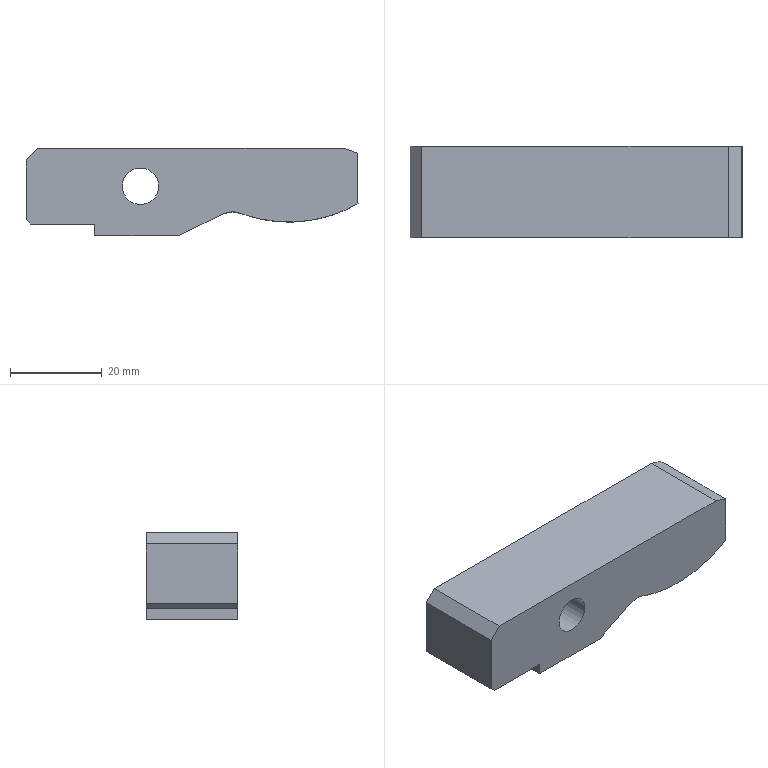Part | 1 solid | 14 faces | box 72.5 x 20 x 19 mm | volume 22819 mm3 | plane 11 | cylinder 2 | other 1 | commonest cylinder face diameters 8 x2
STEP:
#1=CARTESIAN_POINT('',(0.,0.,0.));
#2=DIRECTION('',(0.,0.,1.));
#3=DIRECTION('',(1.,0.,0.));
#4=AXIS2_PLACEMENT_3D('',#1,#2,#3);
#5=CARTESIAN_POINT('',(-58.53,150.526,-242.362));
#6=VERTEX_POINT('',#5);
#7=CARTESIAN_POINT('',(-58.53,150.526,-231.349));
#8=VERTEX_POINT('',#7);
#9=CARTESIAN_POINT('',(-58.53,150.526,-242.362));
#10=DIRECTION('',(-0.000000001,0.,1.));
#11=VECTOR('',#10,1.);
#12=LINE('',#9,#11);
#13=CARTESIAN_POINT('',(-58.53,130.526,-242.362));
#14=DIRECTION('',(-1.,0.,-0.000000001));
#15=DIRECTION('',(0.000000001,0.,-1.));
#16=AXIS2_PLACEMENT_3D('',#13,#14,#15);
#17=PLANE('',#16);
#18=CARTESIAN_POINT('',(0.,-20.));
#19=DIRECTION('',(-1.,0.));
#20=VECTOR('',#19,1.);
#21=LINE('',#18,#20);
#22=(GEOMETRIC_REPRESENTATION_CONTEXT(2)PARAMETRIC_REPRESENTATION_CONTEXT()REPRESENTATION_CONTEXT('',''));
#23=DEFINITIONAL_REPRESENTATION('',(#21),#22);
#24=PCURVE('',#17,#23);
#25=CARTESIAN_POINT('',(-77.88,150.526,-246.104));
#26=DIRECTION('',(0.,-1.,0.));
#27=DIRECTION('',(1.,0.,0.));
#28=AXIS2_PLACEMENT_3D('',#25,#26,#27);
#29=PLANE('',#28);
#30=CARTESIAN_POINT('',(19.35,3.742));
#31=DIRECTION('',(-0.000000001,1.));
#32=VECTOR('',#31,1.);
#33=LINE('',#30,#32);
#34=(GEOMETRIC_REPRESENTATION_CONTEXT(2)PARAMETRIC_REPRESENTATION_CONTEXT()REPRESENTATION_CONTEXT('',''));
#35=DEFINITIONAL_REPRESENTATION('',(#33),#34);
#36=PCURVE('',#29,#35);
#37=SURFACE_CURVE('',#12,(#24,#36),.PCURVE_S1.);
#38=EDGE_CURVE('',#6,#8,#37,.T.);
#39=ORIENTED_EDGE('',*,*,#38,.T.);
#40=CARTESIAN_POINT('',(-58.53,130.526,-231.349));
#41=VERTEX_POINT('',#40);
#42=CARTESIAN_POINT('',(-58.53,130.526,-231.349));
#43=DIRECTION('',(0.,1.,0.));
#44=VECTOR('',#43,1.);
#45=LINE('',#42,#44);
#46=CARTESIAN_POINT('',(-11.013,0.));
#47=DIRECTION('',(0.,-1.));
#48=VECTOR('',#47,1.);
#49=LINE('',#46,#48);
#50=(GEOMETRIC_REPRESENTATION_CONTEXT(2)PARAMETRIC_REPRESENTATION_CONTEXT()REPRESENTATION_CONTEXT('',''));
#51=DEFINITIONAL_REPRESENTATION('',(#49),#50);
#52=PCURVE('',#17,#51);
#53=CARTESIAN_POINT('',(-58.53,130.526,-231.349));
#54=DIRECTION('',(-0.3162,0.,-0.9487));
#55=DIRECTION('',(0.9487,0.,-0.3162));
#56=AXIS2_PLACEMENT_3D('',#53,#54,#55);
#57=PLANE('',#56);
#58=CARTESIAN_POINT('',(0.,0.));
#59=DIRECTION('',(0.,-1.));
#60=VECTOR('',#59,1.);
#61=LINE('',#58,#60);
#62=(GEOMETRIC_REPRESENTATION_CONTEXT(2)PARAMETRIC_REPRESENTATION_CONTEXT()REPRESENTATION_CONTEXT('',''));
#63=DEFINITIONAL_REPRESENTATION('',(#61),#62);
#64=PCURVE('',#57,#63);
#65=SURFACE_CURVE('',#45,(#52,#64),.PCURVE_S1.);
#66=EDGE_CURVE('',#41,#8,#65,.T.);
#67=ORIENTED_EDGE('',*,*,#66,.F.);
#68=CARTESIAN_POINT('',(-58.53,130.526,-242.362));
#69=VERTEX_POINT('',#68);
#70=CARTESIAN_POINT('',(-58.53,130.526,-242.362));
#71=DIRECTION('',(-0.000000001,0.,1.));
#72=VECTOR('',#71,1.);
#73=LINE('',#70,#72);
#74=CARTESIAN_POINT('',(0.,0.));
#75=DIRECTION('',(-1.,0.));
#76=VECTOR('',#75,1.);
#77=LINE('',#74,#76);
#78=(GEOMETRIC_REPRESENTATION_CONTEXT(2)PARAMETRIC_REPRESENTATION_CONTEXT()REPRESENTATION_CONTEXT('',''));
#79=DEFINITIONAL_REPRESENTATION('',(#77),#78);
#80=PCURVE('',#17,#79);
#81=CARTESIAN_POINT('',(-77.88,130.526,-246.104));
#82=DIRECTION('',(0.,-1.,0.));
#83=DIRECTION('',(1.,0.,0.));
#84=AXIS2_PLACEMENT_3D('',#81,#82,#83);
#85=PLANE('',#84);
#86=CARTESIAN_POINT('',(19.35,3.742));
#87=DIRECTION('',(-0.000000001,1.));
#88=VECTOR('',#87,1.);
#89=LINE('',#86,#88);
#90=(GEOMETRIC_REPRESENTATION_CONTEXT(2)PARAMETRIC_REPRESENTATION_CONTEXT()REPRESENTATION_CONTEXT('',''));
#91=DEFINITIONAL_REPRESENTATION('',(#89),#90);
#92=PCURVE('',#85,#91);
#93=SURFACE_CURVE('',#73,(#80,#92),.PCURVE_S1.);
#94=EDGE_CURVE('',#69,#41,#93,.T.);
#95=ORIENTED_EDGE('',*,*,#94,.F.);
#96=CARTESIAN_POINT('',(-58.53,130.526,-242.362));
#97=DIRECTION('',(0.,1.,0.));
#98=VECTOR('',#97,1.);
#99=LINE('',#96,#98);
#100=CARTESIAN_POINT('',(0.,0.));
#101=DIRECTION('',(0.,-1.));
#102=VECTOR('',#101,1.);
#103=LINE('',#100,#102);
#104=(GEOMETRIC_REPRESENTATION_CONTEXT(2)PARAMETRIC_REPRESENTATION_CONTEXT()REPRESENTATION_CONTEXT('',''));
#105=DEFINITIONAL_REPRESENTATION('',(#103),#104);
#106=PCURVE('',#17,#105);
#107=CARTESIAN_POINT('',(-97.53,130.526,-249.349));
#108=CARTESIAN_POINT('',(-94.389,130.526,-247.793));
#109=CARTESIAN_POINT('',(-91.248,130.526,-246.237));
#110=CARTESIAN_POINT('',(-88.106,130.526,-244.681));
#111=CARTESIAN_POINT('',(-86.843,130.526,-244.055));
#112=CARTESIAN_POINT('',(-85.434,130.526,-243.986));
#113=CARTESIAN_POINT('',(-84.116,130.526,-244.486));
#114=CARTESIAN_POINT('',(-75.557,130.526,-247.728));
#115=CARTESIAN_POINT('',(-66.437,130.526,-246.971));
#116=CARTESIAN_POINT('',(-58.53,130.526,-242.362));
#117=(BOUNDED_CURVE()B_SPLINE_CURVE(3,(#107,#108,#109,#110,#111,#112,#113,#114,#115,#116),.UNSPECIFIED.,.F.,.F.)B_SPLINE_CURVE_WITH_KNOTS((4,3,3,4),(0.,2.492,3.494,10.),.UNSPECIFIED.)CURVE()GEOMETRIC_REPRESENTATION_ITEM()RATIONAL_B_SPLINE_CURVE((0.5256,0.5256,0.5256,0.5256,0.4964,0.4964,0.5256,0.4915,0.4915,0.5256))REPRESENTATION_ITEM(''));
#118=DIRECTION('',(0.,1.,0.));
#119=VECTOR('',#118,1.);
#120=SURFACE_OF_LINEAR_EXTRUSION('',#117,#119);
#121=CARTESIAN_POINT('',(10.,0.));
#122=DIRECTION('',(0.,1.));
#123=VECTOR('',#122,1.);
#124=LINE('',#121,#123);
#125=(GEOMETRIC_REPRESENTATION_CONTEXT(2)PARAMETRIC_REPRESENTATION_CONTEXT()REPRESENTATION_CONTEXT('',''));
#126=DEFINITIONAL_REPRESENTATION('',(#124),#125);
#127=PCURVE('',#120,#126);
#128=SURFACE_CURVE('',#99,(#106,#127),.PCURVE_S1.);
#129=EDGE_CURVE('',#69,#6,#128,.T.);
#130=ORIENTED_EDGE('',*,*,#129,.T.);
#131=EDGE_LOOP('',(#39,#67,#95,#130));
#132=FACE_BOUND('',#131,.T.);
#133=ADVANCED_FACE('',(#132),#17,.F.);
#134=CARTESIAN_POINT('',(-97.53,130.526,-249.349));
#135=VERTEX_POINT('',#134);
#136=CARTESIAN_POINT('',(-97.53,150.526,-249.349));
#137=VERTEX_POINT('',#136);
#138=CARTESIAN_POINT('',(-97.53,130.526,-249.349));
#139=DIRECTION('',(0.,1.,0.));
#140=VECTOR('',#139,1.);
#141=LINE('',#138,#140);
#142=CARTESIAN_POINT('',(0.,0.));
#143=DIRECTION('',(0.,1.));
#144=VECTOR('',#143,1.);
#145=LINE('',#142,#144);
#146=(GEOMETRIC_REPRESENTATION_CONTEXT(2)PARAMETRIC_REPRESENTATION_CONTEXT()REPRESENTATION_CONTEXT('',''));
#147=DEFINITIONAL_REPRESENTATION('',(#145),#146);
#148=PCURVE('',#120,#147);
#149=CARTESIAN_POINT('',(-116.03,130.526,-249.349));
#150=DIRECTION('',(0.,0.,1.));
#151=DIRECTION('',(0.,-1.,0.));
#152=AXIS2_PLACEMENT_3D('',#149,#150,#151);
#153=PLANE('',#152);
#154=CARTESIAN_POINT('',(0.,18.5));
#155=DIRECTION('',(-1.,0.));
#156=VECTOR('',#155,1.);
#157=LINE('',#154,#156);
#158=(GEOMETRIC_REPRESENTATION_CONTEXT(2)PARAMETRIC_REPRESENTATION_CONTEXT()REPRESENTATION_CONTEXT('',''));
#159=DEFINITIONAL_REPRESENTATION('',(#157),#158);
#160=PCURVE('',#153,#159);
#161=SURFACE_CURVE('',#141,(#148,#160),.PCURVE_S1.);
#162=EDGE_CURVE('',#135,#137,#161,.T.);
#163=ORIENTED_EDGE('',*,*,#162,.F.);
#164=CARTESIAN_POINT('',(-97.53,130.526,-249.349));
#165=CARTESIAN_POINT('',(-94.389,130.526,-247.793));
#166=CARTESIAN_POINT('',(-91.248,130.526,-246.237));
#167=CARTESIAN_POINT('',(-88.106,130.526,-244.681));
#168=CARTESIAN_POINT('',(-86.843,130.526,-244.055));
#169=CARTESIAN_POINT('',(-85.434,130.526,-243.986));
#170=CARTESIAN_POINT('',(-84.116,130.526,-244.486));
#171=CARTESIAN_POINT('',(-75.557,130.526,-247.728));
#172=CARTESIAN_POINT('',(-66.437,130.526,-246.971));
#173=CARTESIAN_POINT('',(-58.53,130.526,-242.362));
#174=(BOUNDED_CURVE()B_SPLINE_CURVE(3,(#164,#165,#166,#167,#168,#169,#170,#171,#172,#173),.UNSPECIFIED.,.F.,.F.)B_SPLINE_CURVE_WITH_KNOTS((4,3,3,4),(0.,10.129,14.203,42.203),.UNSPECIFIED.)CURVE()GEOMETRIC_REPRESENTATION_ITEM()RATIONAL_B_SPLINE_CURVE((0.5256,0.5256,0.5256,0.5256,0.4964,0.4964,0.5256,0.4915,0.4915,0.5256))REPRESENTATION_ITEM(''));
#175=CARTESIAN_POINT('',(0.,0.));
#176=CARTESIAN_POINT('',(0.1573,0.));
#177=CARTESIAN_POINT('',(0.4719,0.));
#178=CARTESIAN_POINT('',(0.9439,0.));
#179=CARTESIAN_POINT('',(1.416,0.));
#180=CARTESIAN_POINT('',(1.888,0.));
#181=CARTESIAN_POINT('',(2.36,0.));
#182=CARTESIAN_POINT('',(2.831,0.));
#183=CARTESIAN_POINT('',(3.307,0.));
#184=CARTESIAN_POINT('',(3.762,0.));
#185=CARTESIAN_POINT('',(4.205,0.));
#186=CARTESIAN_POINT('',(4.651,0.));
#187=CARTESIAN_POINT('',(5.097,0.));
#188=CARTESIAN_POINT('',(5.543,0.));
#189=CARTESIAN_POINT('',(5.988,0.));
#190=CARTESIAN_POINT('',(6.434,0.));
#191=CARTESIAN_POINT('',(6.88,0.));
#192=CARTESIAN_POINT('',(7.326,0.));
#193=CARTESIAN_POINT('',(7.771,0.));
#194=CARTESIAN_POINT('',(8.217,0.));
#195=CARTESIAN_POINT('',(8.663,0.));
#196=CARTESIAN_POINT('',(9.109,0.));
#197=CARTESIAN_POINT('',(9.554,0.));
#198=CARTESIAN_POINT('',(9.851,0.));
#199=CARTESIAN_POINT('',(10.,0.));
#200=B_SPLINE_CURVE_WITH_KNOTS('',3,(#175,#176,#177,#178,#179,#180,#181,#182,#183,#184,#185,#186,#187,#188,#189,#190,#191,#192,#193,#194,#195,#196,#197,#198,#199),.UNSPECIFIED.,.F.,.F.,(4,1,1,1,1,1,1,1,1,1,1,1,1,1,1,1,1,1,1,1,1,1,4),(0.,1.918,3.837,5.755,7.673,9.592,11.51,13.428,15.346,17.265,19.183,21.101,23.02,24.938,26.856,28.775,30.693,32.611,34.529,36.448,38.366,40.284,42.203),.QUASI_UNIFORM_KNOTS.);
#201=(GEOMETRIC_REPRESENTATION_CONTEXT(2)PARAMETRIC_REPRESENTATION_CONTEXT()REPRESENTATION_CONTEXT('',''));
#202=DEFINITIONAL_REPRESENTATION('',(#200),#201);
#203=PCURVE('',#120,#202);
#204=CARTESIAN_POINT('',(-19.65,-3.245));
#205=CARTESIAN_POINT('',(-16.509,-1.689));
#206=CARTESIAN_POINT('',(-13.368,-0.1328));
#207=CARTESIAN_POINT('',(-10.227,1.423));
#208=CARTESIAN_POINT('',(-8.963,2.049));
#209=CARTESIAN_POINT('',(-7.555,2.118));
#210=CARTESIAN_POINT('',(-6.236,1.618));
#211=CARTESIAN_POINT('',(2.322,-1.624));
#212=CARTESIAN_POINT('',(11.443,-0.867));
#213=CARTESIAN_POINT('',(19.35,3.742));
#214=(BOUNDED_CURVE()B_SPLINE_CURVE(3,(#204,#205,#206,#207,#208,#209,#210,#211,#212,#213),.UNSPECIFIED.,.F.,.F.)B_SPLINE_CURVE_WITH_KNOTS((4,3,3,4),(0.,10.129,14.203,42.203),.UNSPECIFIED.)CURVE()GEOMETRIC_REPRESENTATION_ITEM()RATIONAL_B_SPLINE_CURVE((0.5256,0.5256,0.5256,0.5256,0.4964,0.4964,0.5256,0.4915,0.4915,0.5256))REPRESENTATION_ITEM(''));
#215=(GEOMETRIC_REPRESENTATION_CONTEXT(2)PARAMETRIC_REPRESENTATION_CONTEXT()REPRESENTATION_CONTEXT('',''));
#216=DEFINITIONAL_REPRESENTATION('',(#214),#215);
#217=PCURVE('',#85,#216);
#218=SURFACE_CURVE('',#174,(#203,#217),.PCURVE_S1.);
#219=EDGE_CURVE('',#135,#69,#218,.T.);
#220=ORIENTED_EDGE('',*,*,#219,.T.);
#221=ORIENTED_EDGE('',*,*,#129,.T.);
#222=CARTESIAN_POINT('',(-97.53,150.526,-249.349));
#223=CARTESIAN_POINT('',(-94.389,150.526,-247.793));
#224=CARTESIAN_POINT('',(-91.248,150.526,-246.237));
#225=CARTESIAN_POINT('',(-88.106,150.526,-244.681));
#226=CARTESIAN_POINT('',(-86.843,150.526,-244.055));
#227=CARTESIAN_POINT('',(-85.434,150.526,-243.986));
#228=CARTESIAN_POINT('',(-84.116,150.526,-244.486));
#229=CARTESIAN_POINT('',(-75.557,150.526,-247.728));
#230=CARTESIAN_POINT('',(-66.437,150.526,-246.971));
#231=CARTESIAN_POINT('',(-58.53,150.526,-242.362));
#232=(BOUNDED_CURVE()B_SPLINE_CURVE(3,(#222,#223,#224,#225,#226,#227,#228,#229,#230,#231),.UNSPECIFIED.,.F.,.F.)B_SPLINE_CURVE_WITH_KNOTS((4,3,3,4),(0.,10.129,14.203,42.203),.UNSPECIFIED.)CURVE()GEOMETRIC_REPRESENTATION_ITEM()RATIONAL_B_SPLINE_CURVE((0.5256,0.5256,0.5256,0.5256,0.4964,0.4964,0.5256,0.4915,0.4915,0.5256))REPRESENTATION_ITEM(''));
#233=CARTESIAN_POINT('',(0.,20.));
#234=CARTESIAN_POINT('',(0.1573,20.));
#235=CARTESIAN_POINT('',(0.4719,20.));
#236=CARTESIAN_POINT('',(0.9439,20.));
#237=CARTESIAN_POINT('',(1.416,20.));
#238=CARTESIAN_POINT('',(1.888,20.));
#239=CARTESIAN_POINT('',(2.36,20.));
#240=CARTESIAN_POINT('',(2.831,20.));
#241=CARTESIAN_POINT('',(3.307,20.));
#242=CARTESIAN_POINT('',(3.762,20.));
#243=CARTESIAN_POINT('',(4.205,20.));
#244=CARTESIAN_POINT('',(4.651,20.));
#245=CARTESIAN_POINT('',(5.097,20.));
#246=CARTESIAN_POINT('',(5.543,20.));
#247=CARTESIAN_POINT('',(5.988,20.));
#248=CARTESIAN_POINT('',(6.434,20.));
#249=CARTESIAN_POINT('',(6.88,20.));
#250=CARTESIAN_POINT('',(7.326,20.));
#251=CARTESIAN_POINT('',(7.771,20.));
#252=CARTESIAN_POINT('',(8.217,20.));
#253=CARTESIAN_POINT('',(8.663,20.));
#254=CARTESIAN_POINT('',(9.109,20.));
#255=CARTESIAN_POINT('',(9.554,20.));
#256=CARTESIAN_POINT('',(9.851,20.));
#257=CARTESIAN_POINT('',(10.,20.));
#258=B_SPLINE_CURVE_WITH_KNOTS('',3,(#233,#234,#235,#236,#237,#238,#239,#240,#241,#242,#243,#244,#245,#246,#247,#248,#249,#250,#251,#252,#253,#254,#255,#256,#257),.UNSPECIFIED.,.F.,.F.,(4,1,1,1,1,1,1,1,1,1,1,1,1,1,1,1,1,1,1,1,1,1,4),(0.,1.918,3.837,5.755,7.673,9.592,11.51,13.428,15.346,17.265,19.183,21.101,23.02,24.938,26.856,28.775,30.693,32.611,34.529,36.448,38.366,40.284,42.203),.QUASI_UNIFORM_KNOTS.);
#259=(GEOMETRIC_REPRESENTATION_CONTEXT(2)PARAMETRIC_REPRESENTATION_CONTEXT()REPRESENTATION_CONTEXT('',''));
#260=DEFINITIONAL_REPRESENTATION('',(#258),#259);
#261=PCURVE('',#120,#260);
#262=CARTESIAN_POINT('',(-19.65,-3.245));
#263=CARTESIAN_POINT('',(-16.509,-1.689));
#264=CARTESIAN_POINT('',(-13.368,-0.1328));
#265=CARTESIAN_POINT('',(-10.227,1.423));
#266=CARTESIAN_POINT('',(-8.963,2.049));
#267=CARTESIAN_POINT('',(-7.555,2.118));
#268=CARTESIAN_POINT('',(-6.236,1.618));
#269=CARTESIAN_POINT('',(2.322,-1.624));
#270=CARTESIAN_POINT('',(11.443,-0.867));
#271=CARTESIAN_POINT('',(19.35,3.742));
#272=(BOUNDED_CURVE()B_SPLINE_CURVE(3,(#262,#263,#264,#265,#266,#267,#268,#269,#270,#271),.UNSPECIFIED.,.F.,.F.)B_SPLINE_CURVE_WITH_KNOTS((4,3,3,4),(0.,10.129,14.203,42.203),.UNSPECIFIED.)CURVE()GEOMETRIC_REPRESENTATION_ITEM()RATIONAL_B_SPLINE_CURVE((0.5256,0.5256,0.5256,0.5256,0.4964,0.4964,0.5256,0.4915,0.4915,0.5256))REPRESENTATION_ITEM(''));
#273=(GEOMETRIC_REPRESENTATION_CONTEXT(2)PARAMETRIC_REPRESENTATION_CONTEXT()REPRESENTATION_CONTEXT('',''));
#274=DEFINITIONAL_REPRESENTATION('',(#272),#273);
#275=PCURVE('',#29,#274);
#276=SURFACE_CURVE('',#232,(#261,#275),.PCURVE_S1.);
#277=EDGE_CURVE('',#137,#6,#276,.T.);
#278=ORIENTED_EDGE('',*,*,#277,.F.);
#279=EDGE_LOOP('',(#163,#220,#221,#278));
#280=FACE_BOUND('',#279,.F.);
#281=ADVANCED_FACE('',(#280),#120,.F.);
#282=CARTESIAN_POINT('',(-116.03,150.526,-249.349));
#283=VERTEX_POINT('',#282);
#284=CARTESIAN_POINT('',(-116.03,150.526,-249.349));
#285=DIRECTION('',(1.,0.,0.));
#286=VECTOR('',#285,1.);
#287=LINE('',#284,#286);
#288=CARTESIAN_POINT('',(-20.,0.));
#289=DIRECTION('',(0.,1.));
#290=VECTOR('',#289,1.);
#291=LINE('',#288,#290);
#292=(GEOMETRIC_REPRESENTATION_CONTEXT(2)PARAMETRIC_REPRESENTATION_CONTEXT()REPRESENTATION_CONTEXT('',''));
#293=DEFINITIONAL_REPRESENTATION('',(#291),#292);
#294=PCURVE('',#153,#293);
#295=CARTESIAN_POINT('',(-38.15,-3.245));
#296=DIRECTION('',(1.,0.));
#297=VECTOR('',#296,1.);
#298=LINE('',#295,#297);
#299=(GEOMETRIC_REPRESENTATION_CONTEXT(2)PARAMETRIC_REPRESENTATION_CONTEXT()REPRESENTATION_CONTEXT('',''));
#300=DEFINITIONAL_REPRESENTATION('',(#298),#299);
#301=PCURVE('',#29,#300);
#302=SURFACE_CURVE('',#287,(#294,#301),.PCURVE_S1.);
#303=EDGE_CURVE('',#283,#137,#302,.T.);
#304=ORIENTED_EDGE('',*,*,#303,.T.);
#305=ORIENTED_EDGE('',*,*,#162,.F.);
#306=CARTESIAN_POINT('',(-116.03,130.526,-249.349));
#307=VERTEX_POINT('',#306);
#308=CARTESIAN_POINT('',(-116.03,130.526,-249.349));
#309=DIRECTION('',(1.,0.,0.));
#310=VECTOR('',#309,1.);
#311=LINE('',#308,#310);
#312=CARTESIAN_POINT('',(0.,0.));
#313=DIRECTION('',(0.,1.));
#314=VECTOR('',#313,1.);
#315=LINE('',#312,#314);
#316=(GEOMETRIC_REPRESENTATION_CONTEXT(2)PARAMETRIC_REPRESENTATION_CONTEXT()REPRESENTATION_CONTEXT('',''));
#317=DEFINITIONAL_REPRESENTATION('',(#315),#316);
#318=PCURVE('',#153,#317);
#319=CARTESIAN_POINT('',(-38.15,-3.245));
#320=DIRECTION('',(1.,0.));
#321=VECTOR('',#320,1.);
#322=LINE('',#319,#321);
#323=(GEOMETRIC_REPRESENTATION_CONTEXT(2)PARAMETRIC_REPRESENTATION_CONTEXT()REPRESENTATION_CONTEXT('',''));
#324=DEFINITIONAL_REPRESENTATION('',(#322),#323);
#325=PCURVE('',#85,#324);
#326=SURFACE_CURVE('',#311,(#318,#325),.PCURVE_S1.);
#327=EDGE_CURVE('',#307,#135,#326,.T.);
#328=ORIENTED_EDGE('',*,*,#327,.F.);
#329=CARTESIAN_POINT('',(-116.03,130.526,-249.349));
#330=DIRECTION('',(0.,1.,0.));
#331=VECTOR('',#330,1.);
#332=LINE('',#329,#331);
#333=CARTESIAN_POINT('',(0.,0.));
#334=DIRECTION('',(-1.,0.));
#335=VECTOR('',#334,1.);
#336=LINE('',#333,#335);
#337=(GEOMETRIC_REPRESENTATION_CONTEXT(2)PARAMETRIC_REPRESENTATION_CONTEXT()REPRESENTATION_CONTEXT('',''));
#338=DEFINITIONAL_REPRESENTATION('',(#336),#337);
#339=PCURVE('',#153,#338);
#340=CARTESIAN_POINT('',(-116.03,130.526,-246.849));
#341=DIRECTION('',(1.,0.,0.));
#342=DIRECTION('',(0.,0.,1.));
#343=AXIS2_PLACEMENT_3D('',#340,#341,#342);
#344=PLANE('',#343);
#345=CARTESIAN_POINT('',(-2.5,0.));
#346=DIRECTION('',(0.,-1.));
#347=VECTOR('',#346,1.);
#348=LINE('',#345,#347);
#349=(GEOMETRIC_REPRESENTATION_CONTEXT(2)PARAMETRIC_REPRESENTATION_CONTEXT()REPRESENTATION_CONTEXT('',''));
#350=DEFINITIONAL_REPRESENTATION('',(#348),#349);
#351=PCURVE('',#344,#350);
#352=SURFACE_CURVE('',#332,(#339,#351),.PCURVE_S1.);
#353=EDGE_CURVE('',#307,#283,#352,.T.);
#354=ORIENTED_EDGE('',*,*,#353,.T.);
#355=EDGE_LOOP('',(#304,#305,#328,#354));
#356=FACE_BOUND('',#355,.T.);
#357=ADVANCED_FACE('',(#356),#153,.F.);
#358=CARTESIAN_POINT('',(-116.03,150.526,-246.849));
#359=VERTEX_POINT('',#358);
#360=CARTESIAN_POINT('',(-116.03,150.526,-246.849));
#361=DIRECTION('',(0.,0.,-1.));
#362=VECTOR('',#361,1.);
#363=LINE('',#360,#362);
#364=CARTESIAN_POINT('',(0.,-20.));
#365=DIRECTION('',(-1.,0.));
#366=VECTOR('',#365,1.);
#367=LINE('',#364,#366);
#368=(GEOMETRIC_REPRESENTATION_CONTEXT(2)PARAMETRIC_REPRESENTATION_CONTEXT()REPRESENTATION_CONTEXT('',''));
#369=DEFINITIONAL_REPRESENTATION('',(#367),#368);
#370=PCURVE('',#344,#369);
#371=CARTESIAN_POINT('',(-38.15,-0.7447));
#372=DIRECTION('',(0.,-1.));
#373=VECTOR('',#372,1.);
#374=LINE('',#371,#373);
#375=(GEOMETRIC_REPRESENTATION_CONTEXT(2)PARAMETRIC_REPRESENTATION_CONTEXT()REPRESENTATION_CONTEXT('',''));
#376=DEFINITIONAL_REPRESENTATION('',(#374),#375);
#377=PCURVE('',#29,#376);
#378=SURFACE_CURVE('',#363,(#370,#377),.PCURVE_S1.);
#379=EDGE_CURVE('',#359,#283,#378,.T.);
#380=ORIENTED_EDGE('',*,*,#379,.T.);
#381=ORIENTED_EDGE('',*,*,#353,.F.);
#382=CARTESIAN_POINT('',(-116.03,130.526,-246.849));
#383=VERTEX_POINT('',#382);
#384=CARTESIAN_POINT('',(-116.03,130.526,-246.849));
#385=DIRECTION('',(0.,0.,-1.));
#386=VECTOR('',#385,1.);
#387=LINE('',#384,#386);
#388=CARTESIAN_POINT('',(0.,0.));
#389=DIRECTION('',(-1.,0.));
#390=VECTOR('',#389,1.);
#391=LINE('',#388,#390);
#392=(GEOMETRIC_REPRESENTATION_CONTEXT(2)PARAMETRIC_REPRESENTATION_CONTEXT()REPRESENTATION_CONTEXT('',''));
#393=DEFINITIONAL_REPRESENTATION('',(#391),#392);
#394=PCURVE('',#344,#393);
#395=CARTESIAN_POINT('',(-38.15,-0.7447));
#396=DIRECTION('',(0.,-1.));
#397=VECTOR('',#396,1.);
#398=LINE('',#395,#397);
#399=(GEOMETRIC_REPRESENTATION_CONTEXT(2)PARAMETRIC_REPRESENTATION_CONTEXT()REPRESENTATION_CONTEXT('',''));
#400=DEFINITIONAL_REPRESENTATION('',(#398),#399);
#401=PCURVE('',#85,#400);
#402=SURFACE_CURVE('',#387,(#394,#401),.PCURVE_S1.);
#403=EDGE_CURVE('',#383,#307,#402,.T.);
#404=ORIENTED_EDGE('',*,*,#403,.F.);
#405=CARTESIAN_POINT('',(-116.03,130.526,-246.849));
#406=DIRECTION('',(0.,1.,0.));
#407=VECTOR('',#406,1.);
#408=LINE('',#405,#407);
#409=CARTESIAN_POINT('',(0.,0.));
#410=DIRECTION('',(0.,-1.));
#411=VECTOR('',#410,1.);
#412=LINE('',#409,#411);
#413=(GEOMETRIC_REPRESENTATION_CONTEXT(2)PARAMETRIC_REPRESENTATION_CONTEXT()REPRESENTATION_CONTEXT('',''));
#414=DEFINITIONAL_REPRESENTATION('',(#412),#413);
#415=PCURVE('',#344,#414);
#416=CARTESIAN_POINT('',(-130.03,130.526,-246.849));
#417=DIRECTION('',(0.,0.,1.));
#418=DIRECTION('',(-1.,0.,0.));
#419=AXIS2_PLACEMENT_3D('',#416,#417,#418);
#420=PLANE('',#419);
#421=CARTESIAN_POINT('',(-14.,0.));
#422=DIRECTION('',(0.,-1.));
#423=VECTOR('',#422,1.);
#424=LINE('',#421,#423);
#425=(GEOMETRIC_REPRESENTATION_CONTEXT(2)PARAMETRIC_REPRESENTATION_CONTEXT()REPRESENTATION_CONTEXT('',''));
#426=DEFINITIONAL_REPRESENTATION('',(#424),#425);
#427=PCURVE('',#420,#426);
#428=SURFACE_CURVE('',#408,(#415,#427),.PCURVE_S1.);
#429=EDGE_CURVE('',#383,#359,#428,.T.);
#430=ORIENTED_EDGE('',*,*,#429,.T.);
#431=EDGE_LOOP('',(#380,#381,#404,#430));
#432=FACE_BOUND('',#431,.T.);
#433=ADVANCED_FACE('',(#432),#344,.F.);
#434=CARTESIAN_POINT('',(-130.03,150.526,-246.849));
#435=VERTEX_POINT('',#434);
#436=CARTESIAN_POINT('',(-130.03,150.526,-246.849));
#437=DIRECTION('',(1.,0.,0.));
#438=VECTOR('',#437,1.);
#439=LINE('',#436,#438);
#440=CARTESIAN_POINT('',(0.,-20.));
#441=DIRECTION('',(-1.,0.));
#442=VECTOR('',#441,1.);
#443=LINE('',#440,#442);
#444=(GEOMETRIC_REPRESENTATION_CONTEXT(2)PARAMETRIC_REPRESENTATION_CONTEXT()REPRESENTATION_CONTEXT('',''));
#445=DEFINITIONAL_REPRESENTATION('',(#443),#444);
#446=PCURVE('',#420,#445);
#447=CARTESIAN_POINT('',(-52.15,-0.7447));
#448=DIRECTION('',(1.,0.));
#449=VECTOR('',#448,1.);
#450=LINE('',#447,#449);
#451=(GEOMETRIC_REPRESENTATION_CONTEXT(2)PARAMETRIC_REPRESENTATION_CONTEXT()REPRESENTATION_CONTEXT('',''));
#452=DEFINITIONAL_REPRESENTATION('',(#450),#451);
#453=PCURVE('',#29,#452);
#454=SURFACE_CURVE('',#439,(#446,#453),.PCURVE_S1.);
#455=EDGE_CURVE('',#435,#359,#454,.T.);
#456=ORIENTED_EDGE('',*,*,#455,.T.);
#457=ORIENTED_EDGE('',*,*,#429,.F.);
#458=CARTESIAN_POINT('',(-130.03,130.526,-246.849));
#459=VERTEX_POINT('',#458);
#460=CARTESIAN_POINT('',(-130.03,130.526,-246.849));
#461=DIRECTION('',(1.,0.,0.));
#462=VECTOR('',#461,1.);
#463=LINE('',#460,#462);
#464=CARTESIAN_POINT('',(0.,0.));
#465=DIRECTION('',(-1.,0.));
#466=VECTOR('',#465,1.);
#467=LINE('',#464,#466);
#468=(GEOMETRIC_REPRESENTATION_CONTEXT(2)PARAMETRIC_REPRESENTATION_CONTEXT()REPRESENTATION_CONTEXT('',''));
#469=DEFINITIONAL_REPRESENTATION('',(#467),#468);
#470=PCURVE('',#420,#469);
#471=CARTESIAN_POINT('',(-52.15,-0.7447));
#472=DIRECTION('',(1.,0.));
#473=VECTOR('',#472,1.);
#474=LINE('',#471,#473);
#475=(GEOMETRIC_REPRESENTATION_CONTEXT(2)PARAMETRIC_REPRESENTATION_CONTEXT()REPRESENTATION_CONTEXT('',''));
#476=DEFINITIONAL_REPRESENTATION('',(#474),#475);
#477=PCURVE('',#85,#476);
#478=SURFACE_CURVE('',#463,(#470,#477),.PCURVE_S1.);
#479=EDGE_CURVE('',#459,#383,#478,.T.);
#480=ORIENTED_EDGE('',*,*,#479,.F.);
#481=CARTESIAN_POINT('',(-130.03,130.526,-246.849));
#482=DIRECTION('',(0.,1.,0.));
#483=VECTOR('',#482,1.);
#484=LINE('',#481,#483);
#485=CARTESIAN_POINT('',(0.,0.));
#486=DIRECTION('',(0.,-1.));
#487=VECTOR('',#486,1.);
#488=LINE('',#485,#487);
#489=(GEOMETRIC_REPRESENTATION_CONTEXT(2)PARAMETRIC_REPRESENTATION_CONTEXT()REPRESENTATION_CONTEXT('',''));
#490=DEFINITIONAL_REPRESENTATION('',(#488),#489);
#491=PCURVE('',#420,#490);
#492=CARTESIAN_POINT('',(-131.03,130.526,-245.849));
#493=DIRECTION('',(0.7071,0.,0.7071));
#494=DIRECTION('',(-0.7071,0.,0.7071));
#495=AXIS2_PLACEMENT_3D('',#492,#493,#494);
#496=PLANE('',#495);
#497=CARTESIAN_POINT('',(-1.414,0.));
#498=DIRECTION('',(0.,-1.));
#499=VECTOR('',#498,1.);
#500=LINE('',#497,#499);
#501=(GEOMETRIC_REPRESENTATION_CONTEXT(2)PARAMETRIC_REPRESENTATION_CONTEXT()REPRESENTATION_CONTEXT('',''));
#502=DEFINITIONAL_REPRESENTATION('',(#500),#501);
#503=PCURVE('',#496,#502);
#504=SURFACE_CURVE('',#484,(#491,#503),.PCURVE_S1.);
#505=EDGE_CURVE('',#459,#435,#504,.T.);
#506=ORIENTED_EDGE('',*,*,#505,.T.);
#507=EDGE_LOOP('',(#456,#457,#480,#506));
#508=FACE_BOUND('',#507,.T.);
#509=ADVANCED_FACE('',(#508),#420,.F.);
#510=CARTESIAN_POINT('',(-131.03,150.526,-245.849));
#511=VERTEX_POINT('',#510);
#512=CARTESIAN_POINT('',(-131.03,150.526,-245.849));
#513=DIRECTION('',(0.7071,0.,-0.7071));
#514=VECTOR('',#513,1.);
#515=LINE('',#512,#514);
#516=CARTESIAN_POINT('',(0.,-20.));
#517=DIRECTION('',(-1.,0.));
#518=VECTOR('',#517,1.);
#519=LINE('',#516,#518);
#520=(GEOMETRIC_REPRESENTATION_CONTEXT(2)PARAMETRIC_REPRESENTATION_CONTEXT()REPRESENTATION_CONTEXT('',''));
#521=DEFINITIONAL_REPRESENTATION('',(#519),#520);
#522=PCURVE('',#496,#521);
#523=CARTESIAN_POINT('',(-53.15,0.2553));
#524=DIRECTION('',(0.7071,-0.7071));
#525=VECTOR('',#524,1.);
#526=LINE('',#523,#525);
#527=(GEOMETRIC_REPRESENTATION_CONTEXT(2)PARAMETRIC_REPRESENTATION_CONTEXT()REPRESENTATION_CONTEXT('',''));
#528=DEFINITIONAL_REPRESENTATION('',(#526),#527);
#529=PCURVE('',#29,#528);
#530=SURFACE_CURVE('',#515,(#522,#529),.PCURVE_S1.);
#531=EDGE_CURVE('',#511,#435,#530,.T.);
#532=ORIENTED_EDGE('',*,*,#531,.T.);
#533=ORIENTED_EDGE('',*,*,#505,.F.);
#534=CARTESIAN_POINT('',(-131.03,130.526,-245.849));
#535=VERTEX_POINT('',#534);
#536=CARTESIAN_POINT('',(-131.03,130.526,-245.849));
#537=DIRECTION('',(0.7071,0.,-0.7071));
#538=VECTOR('',#537,1.);
#539=LINE('',#536,#538);
#540=CARTESIAN_POINT('',(0.,0.));
#541=DIRECTION('',(-1.,0.));
#542=VECTOR('',#541,1.);
#543=LINE('',#540,#542);
#544=(GEOMETRIC_REPRESENTATION_CONTEXT(2)PARAMETRIC_REPRESENTATION_CONTEXT()REPRESENTATION_CONTEXT('',''));
#545=DEFINITIONAL_REPRESENTATION('',(#543),#544);
#546=PCURVE('',#496,#545);
#547=CARTESIAN_POINT('',(-53.15,0.2553));
#548=DIRECTION('',(0.7071,-0.7071));
#549=VECTOR('',#548,1.);
#550=LINE('',#547,#549);
#551=(GEOMETRIC_REPRESENTATION_CONTEXT(2)PARAMETRIC_REPRESENTATION_CONTEXT()REPRESENTATION_CONTEXT('',''));
#552=DEFINITIONAL_REPRESENTATION('',(#550),#551);
#553=PCURVE('',#85,#552);
#554=SURFACE_CURVE('',#539,(#546,#553),.PCURVE_S1.);
#555=EDGE_CURVE('',#535,#459,#554,.T.);
#556=ORIENTED_EDGE('',*,*,#555,.F.);
#557=CARTESIAN_POINT('',(-131.03,130.526,-245.849));
#558=DIRECTION('',(0.,1.,0.));
#559=VECTOR('',#558,1.);
#560=LINE('',#557,#559);
#561=CARTESIAN_POINT('',(0.,0.));
#562=DIRECTION('',(0.,-1.));
#563=VECTOR('',#562,1.);
#564=LINE('',#561,#563);
#565=(GEOMETRIC_REPRESENTATION_CONTEXT(2)PARAMETRIC_REPRESENTATION_CONTEXT()REPRESENTATION_CONTEXT('',''));
#566=DEFINITIONAL_REPRESENTATION('',(#564),#565);
#567=PCURVE('',#496,#566);
#568=CARTESIAN_POINT('',(-131.03,130.526,-232.849));
#569=DIRECTION('',(1.,0.,0.));
#570=DIRECTION('',(0.,1.,0.));
#571=AXIS2_PLACEMENT_3D('',#568,#569,#570);
#572=PLANE('',#571);
#573=CARTESIAN_POINT('',(0.,-13.));
#574=DIRECTION('',(1.,0.));
#575=VECTOR('',#574,1.);
#576=LINE('',#573,#575);
#577=(GEOMETRIC_REPRESENTATION_CONTEXT(2)PARAMETRIC_REPRESENTATION_CONTEXT()REPRESENTATION_CONTEXT('',''));
#578=DEFINITIONAL_REPRESENTATION('',(#576),#577);
#579=PCURVE('',#572,#578);
#580=SURFACE_CURVE('',#560,(#567,#579),.PCURVE_S1.);
#581=EDGE_CURVE('',#535,#511,#580,.T.);
#582=ORIENTED_EDGE('',*,*,#581,.T.);
#583=EDGE_LOOP('',(#532,#533,#556,#582));
#584=FACE_BOUND('',#583,.T.);
#585=ADVANCED_FACE('',(#584),#496,.F.);
#586=CARTESIAN_POINT('',(-131.03,150.526,-232.849));
#587=VERTEX_POINT('',#586);
#588=CARTESIAN_POINT('',(-131.03,150.526,-232.849));
#589=DIRECTION('',(0.,0.,-1.));
#590=VECTOR('',#589,1.);
#591=LINE('',#588,#590);
#592=CARTESIAN_POINT('',(20.,0.));
#593=DIRECTION('',(0.,-1.));
#594=VECTOR('',#593,1.);
#595=LINE('',#592,#594);
#596=(GEOMETRIC_REPRESENTATION_CONTEXT(2)PARAMETRIC_REPRESENTATION_CONTEXT()REPRESENTATION_CONTEXT('',''));
#597=DEFINITIONAL_REPRESENTATION('',(#595),#596);
#598=PCURVE('',#572,#597);
#599=CARTESIAN_POINT('',(-53.15,13.255));
#600=DIRECTION('',(0.,-1.));
#601=VECTOR('',#600,1.);
#602=LINE('',#599,#601);
#603=(GEOMETRIC_REPRESENTATION_CONTEXT(2)PARAMETRIC_REPRESENTATION_CONTEXT()REPRESENTATION_CONTEXT('',''));
#604=DEFINITIONAL_REPRESENTATION('',(#602),#603);
#605=PCURVE('',#29,#604);
#606=SURFACE_CURVE('',#591,(#598,#605),.PCURVE_S1.);
#607=EDGE_CURVE('',#587,#511,#606,.T.);
#608=ORIENTED_EDGE('',*,*,#607,.T.);
#609=ORIENTED_EDGE('',*,*,#581,.F.);
#610=CARTESIAN_POINT('',(-131.03,130.526,-232.849));
#611=VERTEX_POINT('',#610);
#612=CARTESIAN_POINT('',(-131.03,130.526,-232.849));
#613=DIRECTION('',(0.,0.,-1.));
#614=VECTOR('',#613,1.);
#615=LINE('',#612,#614);
#616=CARTESIAN_POINT('',(0.,0.));
#617=DIRECTION('',(0.,-1.));
#618=VECTOR('',#617,1.);
#619=LINE('',#616,#618);
#620=(GEOMETRIC_REPRESENTATION_CONTEXT(2)PARAMETRIC_REPRESENTATION_CONTEXT()REPRESENTATION_CONTEXT('',''));
#621=DEFINITIONAL_REPRESENTATION('',(#619),#620);
#622=PCURVE('',#572,#621);
#623=CARTESIAN_POINT('',(-53.15,13.255));
#624=DIRECTION('',(0.,-1.));
#625=VECTOR('',#624,1.);
#626=LINE('',#623,#625);
#627=(GEOMETRIC_REPRESENTATION_CONTEXT(2)PARAMETRIC_REPRESENTATION_CONTEXT()REPRESENTATION_CONTEXT('',''));
#628=DEFINITIONAL_REPRESENTATION('',(#626),#627);
#629=PCURVE('',#85,#628);
#630=SURFACE_CURVE('',#615,(#622,#629),.PCURVE_S1.);
#631=EDGE_CURVE('',#611,#535,#630,.T.);
#632=ORIENTED_EDGE('',*,*,#631,.F.);
#633=CARTESIAN_POINT('',(-131.03,130.526,-232.849));
#634=DIRECTION('',(0.,1.,0.));
#635=VECTOR('',#634,1.);
#636=LINE('',#633,#635);
#637=CARTESIAN_POINT('',(0.,0.));
#638=DIRECTION('',(1.,0.));
#639=VECTOR('',#638,1.);
#640=LINE('',#637,#639);
#641=(GEOMETRIC_REPRESENTATION_CONTEXT(2)PARAMETRIC_REPRESENTATION_CONTEXT()REPRESENTATION_CONTEXT('',''));
#642=DEFINITIONAL_REPRESENTATION('',(#640),#641);
#643=PCURVE('',#572,#642);
#644=CARTESIAN_POINT('',(-128.53,130.526,-230.349));
#645=DIRECTION('',(0.7071,0.,-0.7071));
#646=DIRECTION('',(0.7071,0.,0.7071));
#647=AXIS2_PLACEMENT_3D('',#644,#645,#646);
#648=PLANE('',#647);
#649=CARTESIAN_POINT('',(-3.536,0.));
#650=DIRECTION('',(0.,-1.));
#651=VECTOR('',#650,1.);
#652=LINE('',#649,#651);
#653=(GEOMETRIC_REPRESENTATION_CONTEXT(2)PARAMETRIC_REPRESENTATION_CONTEXT()REPRESENTATION_CONTEXT('',''));
#654=DEFINITIONAL_REPRESENTATION('',(#652),#653);
#655=PCURVE('',#648,#654);
#656=SURFACE_CURVE('',#636,(#643,#655),.PCURVE_S1.);
#657=EDGE_CURVE('',#611,#587,#656,.T.);
#658=ORIENTED_EDGE('',*,*,#657,.T.);
#659=EDGE_LOOP('',(#608,#609,#632,#658));
#660=FACE_BOUND('',#659,.T.);
#661=ADVANCED_FACE('',(#660),#572,.F.);
#662=CARTESIAN_POINT('',(-128.53,150.526,-230.349));
#663=VERTEX_POINT('',#662);
#664=CARTESIAN_POINT('',(-128.53,150.526,-230.349));
#665=DIRECTION('',(-0.7071,0.,-0.7071));
#666=VECTOR('',#665,1.);
#667=LINE('',#664,#666);
#668=CARTESIAN_POINT('',(0.,-20.));
#669=DIRECTION('',(-1.,0.));
#670=VECTOR('',#669,1.);
#671=LINE('',#668,#670);
#672=(GEOMETRIC_REPRESENTATION_CONTEXT(2)PARAMETRIC_REPRESENTATION_CONTEXT()REPRESENTATION_CONTEXT('',''));
#673=DEFINITIONAL_REPRESENTATION('',(#671),#672);
#674=PCURVE('',#648,#673);
#675=CARTESIAN_POINT('',(-50.65,15.755));
#676=DIRECTION('',(-0.7071,-0.7071));
#677=VECTOR('',#676,1.);
#678=LINE('',#675,#677);
#679=(GEOMETRIC_REPRESENTATION_CONTEXT(2)PARAMETRIC_REPRESENTATION_CONTEXT()REPRESENTATION_CONTEXT('',''));
#680=DEFINITIONAL_REPRESENTATION('',(#678),#679);
#681=PCURVE('',#29,#680);
#682=SURFACE_CURVE('',#667,(#674,#681),.PCURVE_S1.);
#683=EDGE_CURVE('',#663,#587,#682,.T.);
#684=ORIENTED_EDGE('',*,*,#683,.T.);
#685=ORIENTED_EDGE('',*,*,#657,.F.);
#686=CARTESIAN_POINT('',(-128.53,130.526,-230.349));
#687=VERTEX_POINT('',#686);
#688=CARTESIAN_POINT('',(-128.53,130.526,-230.349));
#689=DIRECTION('',(-0.7071,0.,-0.7071));
#690=VECTOR('',#689,1.);
#691=LINE('',#688,#690);
#692=CARTESIAN_POINT('',(0.,0.));
#693=DIRECTION('',(-1.,0.));
#694=VECTOR('',#693,1.);
#695=LINE('',#692,#694);
#696=(GEOMETRIC_REPRESENTATION_CONTEXT(2)PARAMETRIC_REPRESENTATION_CONTEXT()REPRESENTATION_CONTEXT('',''));
#697=DEFINITIONAL_REPRESENTATION('',(#695),#696);
#698=PCURVE('',#648,#697);
#699=CARTESIAN_POINT('',(-50.65,15.755));
#700=DIRECTION('',(-0.7071,-0.7071));
#701=VECTOR('',#700,1.);
#702=LINE('',#699,#701);
#703=(GEOMETRIC_REPRESENTATION_CONTEXT(2)PARAMETRIC_REPRESENTATION_CONTEXT()REPRESENTATION_CONTEXT('',''));
#704=DEFINITIONAL_REPRESENTATION('',(#702),#703);
#705=PCURVE('',#85,#704);
#706=SURFACE_CURVE('',#691,(#698,#705),.PCURVE_S1.);
#707=EDGE_CURVE('',#687,#611,#706,.T.);
#708=ORIENTED_EDGE('',*,*,#707,.F.);
#709=CARTESIAN_POINT('',(-128.53,130.526,-230.349));
#710=DIRECTION('',(0.,1.,0.));
#711=VECTOR('',#710,1.);
#712=LINE('',#709,#711);
#713=CARTESIAN_POINT('',(0.,0.));
#714=DIRECTION('',(0.,-1.));
#715=VECTOR('',#714,1.);
#716=LINE('',#713,#715);
#717=(GEOMETRIC_REPRESENTATION_CONTEXT(2)PARAMETRIC_REPRESENTATION_CONTEXT()REPRESENTATION_CONTEXT('',''));
#718=DEFINITIONAL_REPRESENTATION('',(#716),#717);
#719=PCURVE('',#648,#718);
#720=CARTESIAN_POINT('',(-61.53,130.526,-230.349));
#721=DIRECTION('',(0.,0.,-1.));
#722=DIRECTION('',(0.,1.,0.));
#723=AXIS2_PLACEMENT_3D('',#720,#721,#722);
#724=PLANE('',#723);
#725=CARTESIAN_POINT('',(0.,-67.));
#726=DIRECTION('',(1.,0.));
#727=VECTOR('',#726,1.);
#728=LINE('',#725,#727);
#729=(GEOMETRIC_REPRESENTATION_CONTEXT(2)PARAMETRIC_REPRESENTATION_CONTEXT()REPRESENTATION_CONTEXT('',''));
#730=DEFINITIONAL_REPRESENTATION('',(#728),#729);
#731=PCURVE('',#724,#730);
#732=SURFACE_CURVE('',#712,(#719,#731),.PCURVE_S1.);
#733=EDGE_CURVE('',#687,#663,#732,.T.);
#734=ORIENTED_EDGE('',*,*,#733,.T.);
#735=EDGE_LOOP('',(#684,#685,#708,#734));
#736=FACE_BOUND('',#735,.T.);
#737=ADVANCED_FACE('',(#736),#648,.F.);
#738=CARTESIAN_POINT('',(-61.53,150.526,-230.349));
#739=VERTEX_POINT('',#738);
#740=CARTESIAN_POINT('',(-61.53,150.526,-230.349));
#741=DIRECTION('',(-1.,0.,0.));
#742=VECTOR('',#741,1.);
#743=LINE('',#740,#742);
#744=CARTESIAN_POINT('',(20.,0.));
#745=DIRECTION('',(0.,-1.));
#746=VECTOR('',#745,1.);
#747=LINE('',#744,#746);
#748=(GEOMETRIC_REPRESENTATION_CONTEXT(2)PARAMETRIC_REPRESENTATION_CONTEXT()REPRESENTATION_CONTEXT('',''));
#749=DEFINITIONAL_REPRESENTATION('',(#747),#748);
#750=PCURVE('',#724,#749);
#751=CARTESIAN_POINT('',(16.35,15.755));
#752=DIRECTION('',(-1.,0.));
#753=VECTOR('',#752,1.);
#754=LINE('',#751,#753);
#755=(GEOMETRIC_REPRESENTATION_CONTEXT(2)PARAMETRIC_REPRESENTATION_CONTEXT()REPRESENTATION_CONTEXT('',''));
#756=DEFINITIONAL_REPRESENTATION('',(#754),#755);
#757=PCURVE('',#29,#756);
#758=SURFACE_CURVE('',#743,(#750,#757),.PCURVE_S1.);
#759=EDGE_CURVE('',#739,#663,#758,.T.);
#760=ORIENTED_EDGE('',*,*,#759,.T.);
#761=ORIENTED_EDGE('',*,*,#733,.F.);
#762=CARTESIAN_POINT('',(-61.53,130.526,-230.349));
#763=VERTEX_POINT('',#762);
#764=CARTESIAN_POINT('',(-61.53,130.526,-230.349));
#765=DIRECTION('',(-1.,0.,0.));
#766=VECTOR('',#765,1.);
#767=LINE('',#764,#766);
#768=CARTESIAN_POINT('',(0.,0.));
#769=DIRECTION('',(0.,-1.));
#770=VECTOR('',#769,1.);
#771=LINE('',#768,#770);
#772=(GEOMETRIC_REPRESENTATION_CONTEXT(2)PARAMETRIC_REPRESENTATION_CONTEXT()REPRESENTATION_CONTEXT('',''));
#773=DEFINITIONAL_REPRESENTATION('',(#771),#772);
#774=PCURVE('',#724,#773);
#775=CARTESIAN_POINT('',(16.35,15.755));
#776=DIRECTION('',(-1.,0.));
#777=VECTOR('',#776,1.);
#778=LINE('',#775,#777);
#779=(GEOMETRIC_REPRESENTATION_CONTEXT(2)PARAMETRIC_REPRESENTATION_CONTEXT()REPRESENTATION_CONTEXT('',''));
#780=DEFINITIONAL_REPRESENTATION('',(#778),#779);
#781=PCURVE('',#85,#780);
#782=SURFACE_CURVE('',#767,(#774,#781),.PCURVE_S1.);
#783=EDGE_CURVE('',#763,#687,#782,.T.);
#784=ORIENTED_EDGE('',*,*,#783,.F.);
#785=CARTESIAN_POINT('',(-61.53,130.526,-230.349));
#786=DIRECTION('',(0.,1.,0.));
#787=VECTOR('',#786,1.);
#788=LINE('',#785,#787);
#789=CARTESIAN_POINT('',(0.,0.));
#790=DIRECTION('',(1.,0.));
#791=VECTOR('',#790,1.);
#792=LINE('',#789,#791);
#793=(GEOMETRIC_REPRESENTATION_CONTEXT(2)PARAMETRIC_REPRESENTATION_CONTEXT()REPRESENTATION_CONTEXT('',''));
#794=DEFINITIONAL_REPRESENTATION('',(#792),#793);
#795=PCURVE('',#724,#794);
#796=CARTESIAN_POINT('',(-3.162,0.));
#797=DIRECTION('',(0.,-1.));
#798=VECTOR('',#797,1.);
#799=LINE('',#796,#798);
#800=(GEOMETRIC_REPRESENTATION_CONTEXT(2)PARAMETRIC_REPRESENTATION_CONTEXT()REPRESENTATION_CONTEXT('',''));
#801=DEFINITIONAL_REPRESENTATION('',(#799),#800);
#802=PCURVE('',#57,#801);
#803=SURFACE_CURVE('',#788,(#795,#802),.PCURVE_S1.);
#804=EDGE_CURVE('',#763,#739,#803,.T.);
#805=ORIENTED_EDGE('',*,*,#804,.T.);
#806=EDGE_LOOP('',(#760,#761,#784,#805));
#807=FACE_BOUND('',#806,.T.);
#808=ADVANCED_FACE('',(#807),#724,.F.);
#809=CARTESIAN_POINT('',(-58.53,150.526,-231.349));
#810=DIRECTION('',(-0.9487,0.,0.3162));
#811=VECTOR('',#810,1.);
#812=LINE('',#809,#811);
#813=CARTESIAN_POINT('',(0.,-20.));
#814=DIRECTION('',(-1.,0.));
#815=VECTOR('',#814,1.);
#816=LINE('',#813,#815);
#817=(GEOMETRIC_REPRESENTATION_CONTEXT(2)PARAMETRIC_REPRESENTATION_CONTEXT()REPRESENTATION_CONTEXT('',''));
#818=DEFINITIONAL_REPRESENTATION('',(#816),#817);
#819=PCURVE('',#57,#818);
#820=CARTESIAN_POINT('',(19.35,14.755));
#821=DIRECTION('',(-0.9487,0.3162));
#822=VECTOR('',#821,1.);
#823=LINE('',#820,#822);
#824=(GEOMETRIC_REPRESENTATION_CONTEXT(2)PARAMETRIC_REPRESENTATION_CONTEXT()REPRESENTATION_CONTEXT('',''));
#825=DEFINITIONAL_REPRESENTATION('',(#823),#824);
#826=PCURVE('',#29,#825);
#827=SURFACE_CURVE('',#812,(#819,#826),.PCURVE_S1.);
#828=EDGE_CURVE('',#8,#739,#827,.T.);
#829=ORIENTED_EDGE('',*,*,#828,.T.);
#830=ORIENTED_EDGE('',*,*,#804,.F.);
#831=CARTESIAN_POINT('',(-58.53,130.526,-231.349));
#832=DIRECTION('',(-0.9487,0.,0.3162));
#833=VECTOR('',#832,1.);
#834=LINE('',#831,#833);
#835=CARTESIAN_POINT('',(0.,0.));
#836=DIRECTION('',(-1.,0.));
#837=VECTOR('',#836,1.);
#838=LINE('',#835,#837);
#839=(GEOMETRIC_REPRESENTATION_CONTEXT(2)PARAMETRIC_REPRESENTATION_CONTEXT()REPRESENTATION_CONTEXT('',''));
#840=DEFINITIONAL_REPRESENTATION('',(#838),#839);
#841=PCURVE('',#57,#840);
#842=CARTESIAN_POINT('',(19.35,14.755));
#843=DIRECTION('',(-0.9487,0.3162));
#844=VECTOR('',#843,1.);
#845=LINE('',#842,#844);
#846=(GEOMETRIC_REPRESENTATION_CONTEXT(2)PARAMETRIC_REPRESENTATION_CONTEXT()REPRESENTATION_CONTEXT('',''));
#847=DEFINITIONAL_REPRESENTATION('',(#845),#846);
#848=PCURVE('',#85,#847);
#849=SURFACE_CURVE('',#834,(#841,#848),.PCURVE_S1.);
#850=EDGE_CURVE('',#41,#763,#849,.T.);
#851=ORIENTED_EDGE('',*,*,#850,.F.);
#852=ORIENTED_EDGE('',*,*,#66,.T.);
#853=EDGE_LOOP('',(#829,#830,#851,#852));
#854=FACE_BOUND('',#853,.T.);
#855=ADVANCED_FACE('',(#854),#57,.F.);
#856=ORIENTED_EDGE('',*,*,#94,.T.);
#857=ORIENTED_EDGE('',*,*,#850,.T.);
#858=ORIENTED_EDGE('',*,*,#783,.T.);
#859=ORIENTED_EDGE('',*,*,#707,.T.);
#860=ORIENTED_EDGE('',*,*,#631,.T.);
#861=ORIENTED_EDGE('',*,*,#555,.T.);
#862=ORIENTED_EDGE('',*,*,#479,.T.);
#863=ORIENTED_EDGE('',*,*,#403,.T.);
#864=ORIENTED_EDGE('',*,*,#327,.T.);
#865=ORIENTED_EDGE('',*,*,#219,.T.);
#866=EDGE_LOOP('',(#856,#857,#858,#859,#860,#861,#862,#863,#864,#865));
#867=FACE_BOUND('',#866,.T.);
#868=CARTESIAN_POINT('',(-102.03,130.526,-238.599));
#869=VERTEX_POINT('',#868);
#870=CARTESIAN_POINT('',(-110.03,130.526,-238.599));
#871=VERTEX_POINT('',#870);
#872=CARTESIAN_POINT('',(-106.03,130.526,-238.599));
#873=DIRECTION('',(0.,-1.,0.));
#874=DIRECTION('',(-1.,0.,0.));
#875=AXIS2_PLACEMENT_3D('',#872,#873,#874);
#876=CIRCLE('',#875,4.);
#877=CARTESIAN_POINT('',(-28.15,7.505));
#878=DIRECTION('',(-1.,0.));
#879=AXIS2_PLACEMENT_2D('',#877,#878);
#880=CIRCLE('',#879,4.);
#881=(GEOMETRIC_REPRESENTATION_CONTEXT(2)PARAMETRIC_REPRESENTATION_CONTEXT()REPRESENTATION_CONTEXT('',''));
#882=DEFINITIONAL_REPRESENTATION('',(#880),#881);
#883=PCURVE('',#85,#882);
#884=CARTESIAN_POINT('',(-106.03,130.526,-238.599));
#885=DIRECTION('',(0.,1.,0.));
#886=DIRECTION('',(0.,0.,-1.));
#887=AXIS2_PLACEMENT_3D('',#884,#885,#886);
#888=CYLINDRICAL_SURFACE('',#887,4.);
#889=CARTESIAN_POINT('',(7.854,0.));
#890=DIRECTION('',(-1.,0.));
#891=VECTOR('',#890,1.);
#892=LINE('',#889,#891);
#893=(GEOMETRIC_REPRESENTATION_CONTEXT(2)PARAMETRIC_REPRESENTATION_CONTEXT()REPRESENTATION_CONTEXT('',''));
#894=DEFINITIONAL_REPRESENTATION('',(#892),#893);
#895=PCURVE('',#888,#894);
#896=SURFACE_CURVE('',#876,(#883,#895),.PCURVE_S1.);
#897=EDGE_CURVE('',#869,#871,#896,.T.);
#898=ORIENTED_EDGE('',*,*,#897,.F.);
#899=CARTESIAN_POINT('',(-106.03,130.526,-238.599));
#900=DIRECTION('',(0.,-1.,0.));
#901=DIRECTION('',(-1.,0.,0.));
#902=AXIS2_PLACEMENT_3D('',#899,#900,#901);
#903=CIRCLE('',#902,4.);
#904=CARTESIAN_POINT('',(-28.15,7.505));
#905=DIRECTION('',(-1.,0.));
#906=AXIS2_PLACEMENT_2D('',#904,#905);
#907=CIRCLE('',#906,4.);
#908=(GEOMETRIC_REPRESENTATION_CONTEXT(2)PARAMETRIC_REPRESENTATION_CONTEXT()REPRESENTATION_CONTEXT('',''));
#909=DEFINITIONAL_REPRESENTATION('',(#907),#908);
#910=PCURVE('',#85,#909);
#911=CARTESIAN_POINT('',(-106.03,130.526,-238.599));
#912=DIRECTION('',(0.,1.,0.));
#913=DIRECTION('',(0.,0.,1.));
#914=AXIS2_PLACEMENT_3D('',#911,#912,#913);
#915=CYLINDRICAL_SURFACE('',#914,4.);
#916=CARTESIAN_POINT('',(4.712,0.));
#917=DIRECTION('',(-1.,0.));
#918=VECTOR('',#917,1.);
#919=LINE('',#916,#918);
#920=(GEOMETRIC_REPRESENTATION_CONTEXT(2)PARAMETRIC_REPRESENTATION_CONTEXT()REPRESENTATION_CONTEXT('',''));
#921=DEFINITIONAL_REPRESENTATION('',(#919),#920);
#922=PCURVE('',#915,#921);
#923=SURFACE_CURVE('',#903,(#910,#922),.PCURVE_S1.);
#924=EDGE_CURVE('',#871,#869,#923,.T.);
#925=ORIENTED_EDGE('',*,*,#924,.F.);
#926=EDGE_LOOP('',(#898,#925));
#927=FACE_BOUND('',#926,.T.);
#928=ADVANCED_FACE('',(#867,#927),#85,.T.);
#929=ORIENTED_EDGE('',*,*,#924,.F.);
#930=CARTESIAN_POINT('',(-110.03,150.526,-238.599));
#931=VERTEX_POINT('',#930);
#932=CARTESIAN_POINT('',(-110.03,130.526,-238.599));
#933=DIRECTION('',(0.,1.,0.));
#934=VECTOR('',#933,1.);
#935=LINE('',#932,#934);
#936=CARTESIAN_POINT('',(4.712,0.));
#937=DIRECTION('',(0.,1.));
#938=VECTOR('',#937,1.);
#939=LINE('',#936,#938);
#940=(GEOMETRIC_REPRESENTATION_CONTEXT(2)PARAMETRIC_REPRESENTATION_CONTEXT()REPRESENTATION_CONTEXT('',''));
#941=DEFINITIONAL_REPRESENTATION('',(#939),#940);
#942=PCURVE('',#915,#941);
#943=CARTESIAN_POINT('',(1.571,0.));
#944=DIRECTION('',(0.,1.));
#945=VECTOR('',#944,1.);
#946=LINE('',#943,#945);
#947=(GEOMETRIC_REPRESENTATION_CONTEXT(2)PARAMETRIC_REPRESENTATION_CONTEXT()REPRESENTATION_CONTEXT('',''));
#948=DEFINITIONAL_REPRESENTATION('',(#946),#947);
#949=PCURVE('',#888,#948);
#950=SURFACE_CURVE('',#935,(#942,#949),.PCURVE_S1.);
#951=EDGE_CURVE('',#871,#931,#950,.T.);
#952=ORIENTED_EDGE('',*,*,#951,.T.);
#953=CARTESIAN_POINT('',(-102.03,150.526,-238.599));
#954=VERTEX_POINT('',#953);
#955=CARTESIAN_POINT('',(-106.03,150.526,-238.599));
#956=DIRECTION('',(0.,-1.,0.));
#957=DIRECTION('',(-1.,0.,0.));
#958=AXIS2_PLACEMENT_3D('',#955,#956,#957);
#959=CIRCLE('',#958,4.);
#960=CARTESIAN_POINT('',(4.712,20.));
#961=DIRECTION('',(-1.,0.));
#962=VECTOR('',#961,1.);
#963=LINE('',#960,#962);
#964=(GEOMETRIC_REPRESENTATION_CONTEXT(2)PARAMETRIC_REPRESENTATION_CONTEXT()REPRESENTATION_CONTEXT('',''));
#965=DEFINITIONAL_REPRESENTATION('',(#963),#964);
#966=PCURVE('',#915,#965);
#967=CARTESIAN_POINT('',(-28.15,7.505));
#968=DIRECTION('',(-1.,0.));
#969=AXIS2_PLACEMENT_2D('',#967,#968);
#970=CIRCLE('',#969,4.);
#971=(GEOMETRIC_REPRESENTATION_CONTEXT(2)PARAMETRIC_REPRESENTATION_CONTEXT()REPRESENTATION_CONTEXT('',''));
#972=DEFINITIONAL_REPRESENTATION('',(#970),#971);
#973=PCURVE('',#29,#972);
#974=SURFACE_CURVE('',#959,(#966,#973),.PCURVE_S1.);
#975=EDGE_CURVE('',#931,#954,#974,.T.);
#976=ORIENTED_EDGE('',*,*,#975,.T.);
#977=CARTESIAN_POINT('',(-102.03,130.526,-238.599));
#978=DIRECTION('',(0.,1.,0.));
#979=VECTOR('',#978,1.);
#980=LINE('',#977,#979);
#981=CARTESIAN_POINT('',(1.571,0.));
#982=DIRECTION('',(0.,1.));
#983=VECTOR('',#982,1.);
#984=LINE('',#981,#983);
#985=(GEOMETRIC_REPRESENTATION_CONTEXT(2)PARAMETRIC_REPRESENTATION_CONTEXT()REPRESENTATION_CONTEXT('',''));
#986=DEFINITIONAL_REPRESENTATION('',(#984),#985);
#987=PCURVE('',#915,#986);
#988=CARTESIAN_POINT('',(4.712,0.));
#989=DIRECTION('',(0.,1.));
#990=VECTOR('',#989,1.);
#991=LINE('',#988,#990);
#992=(GEOMETRIC_REPRESENTATION_CONTEXT(2)PARAMETRIC_REPRESENTATION_CONTEXT()REPRESENTATION_CONTEXT('',''));
#993=DEFINITIONAL_REPRESENTATION('',(#991),#992);
#994=PCURVE('',#888,#993);
#995=SURFACE_CURVE('',#980,(#987,#994),.PCURVE_S1.);
#996=EDGE_CURVE('',#869,#954,#995,.T.);
#997=ORIENTED_EDGE('',*,*,#996,.F.);
#998=EDGE_LOOP('',(#929,#952,#976,#997));
#999=FACE_BOUND('',#998,.F.);
#1000=ADVANCED_FACE('',(#999),#915,.F.);
#1001=ORIENTED_EDGE('',*,*,#38,.F.);
#1002=ORIENTED_EDGE('',*,*,#277,.F.);
#1003=ORIENTED_EDGE('',*,*,#303,.F.);
#1004=ORIENTED_EDGE('',*,*,#379,.F.);
#1005=ORIENTED_EDGE('',*,*,#455,.F.);
#1006=ORIENTED_EDGE('',*,*,#531,.F.);
#1007=ORIENTED_EDGE('',*,*,#607,.F.);
#1008=ORIENTED_EDGE('',*,*,#683,.F.);
#1009=ORIENTED_EDGE('',*,*,#759,.F.);
#1010=ORIENTED_EDGE('',*,*,#828,.F.);
#1011=EDGE_LOOP('',(#1001,#1002,#1003,#1004,#1005,#1006,#1007,#1008,#1009,#1010));
#1012=FACE_BOUND('',#1011,.T.);
#1013=ORIENTED_EDGE('',*,*,#975,.T.);
#1014=CARTESIAN_POINT('',(-106.03,150.526,-238.599));
#1015=DIRECTION('',(0.,-1.,0.));
#1016=DIRECTION('',(-1.,0.,0.));
#1017=AXIS2_PLACEMENT_3D('',#1014,#1015,#1016);
#1018=CIRCLE('',#1017,4.);
#1019=CARTESIAN_POINT('',(-28.15,7.505));
#1020=DIRECTION('',(-1.,0.));
#1021=AXIS2_PLACEMENT_2D('',#1019,#1020);
#1022=CIRCLE('',#1021,4.);
#1023=(GEOMETRIC_REPRESENTATION_CONTEXT(2)PARAMETRIC_REPRESENTATION_CONTEXT()REPRESENTATION_CONTEXT('',''));
#1024=DEFINITIONAL_REPRESENTATION('',(#1022),#1023);
#1025=PCURVE('',#29,#1024);
#1026=CARTESIAN_POINT('',(7.854,20.));
#1027=DIRECTION('',(-1.,0.));
#1028=VECTOR('',#1027,1.);
#1029=LINE('',#1026,#1028);
#1030=(GEOMETRIC_REPRESENTATION_CONTEXT(2)PARAMETRIC_REPRESENTATION_CONTEXT()REPRESENTATION_CONTEXT('',''));
#1031=DEFINITIONAL_REPRESENTATION('',(#1029),#1030);
#1032=PCURVE('',#888,#1031);
#1033=SURFACE_CURVE('',#1018,(#1025,#1032),.PCURVE_S1.);
#1034=EDGE_CURVE('',#954,#931,#1033,.T.);
#1035=ORIENTED_EDGE('',*,*,#1034,.T.);
#1036=EDGE_LOOP('',(#1013,#1035));
#1037=FACE_BOUND('',#1036,.T.);
#1038=ADVANCED_FACE('',(#1012,#1037),#29,.F.);
#1039=ORIENTED_EDGE('',*,*,#1034,.T.);
#1040=ORIENTED_EDGE('',*,*,#951,.F.);
#1041=ORIENTED_EDGE('',*,*,#897,.F.);
#1042=ORIENTED_EDGE('',*,*,#996,.T.);
#1043=EDGE_LOOP('',(#1039,#1040,#1041,#1042));
#1044=FACE_BOUND('',#1043,.F.);
#1045=ADVANCED_FACE('',(#1044),#888,.F.);
#1046=CLOSED_SHELL('',(#133,#281,#357,#433,#509,#585,#661,#737,#808,#855,#928,#1000,#1038,#1045));
#1047=MANIFOLD_SOLID_BREP('',#1046);
#1048=(LENGTH_UNIT()NAMED_UNIT(*)SI_UNIT(.MILLI.,.METRE.));
#1049=UNCERTAINTY_MEASURE_WITH_UNIT(LENGTH_MEASURE(0.0000001),#1048,'','');
#1050=(NAMED_UNIT(*)PLANE_ANGLE_UNIT()SI_UNIT($,.RADIAN.));
#1051=(NAMED_UNIT(*)SI_UNIT($,.STERADIAN.)SOLID_ANGLE_UNIT());
#1052=(GEOMETRIC_REPRESENTATION_CONTEXT(3)GLOBAL_UNCERTAINTY_ASSIGNED_CONTEXT((#1049))GLOBAL_UNIT_ASSIGNED_CONTEXT((#1048,#1050,#1051))REPRESENTATION_CONTEXT('',''));
#1053=ADVANCED_BREP_SHAPE_REPRESENTATION('',(#4,#1047),#1052);